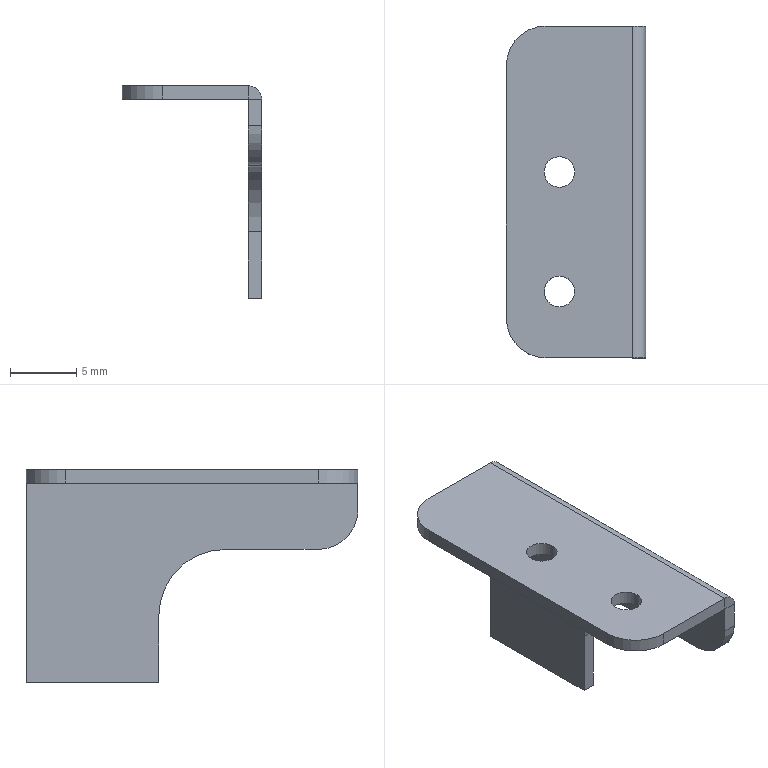Part | SolidWorks | features ICE 2, Fillet 1, FlatPattern 1, SMBaseFlange 1, SheetMetal 1 | 1 solid | 23 faces | box 10.5 x 25 x 16 mm | volume 473.396 mm3 | plane 14 | cylinder 9 | commonest cylinder face diameters 2.3 x4 6 x3 2 x1 10 x1
STEP:
#1=CARTESIAN_POINT('',(-6.65,14.,0.));
#2=VERTEX_POINT('',#1);
#3=CARTESIAN_POINT('',(-4.35,14.,0.));
#4=VERTEX_POINT('',#3);
#5=CARTESIAN_POINT('',(-5.5,14.,0.));
#6=DIRECTION('',(0.,0.,1.));
#7=DIRECTION('',(1.,0.,0.));
#8=AXIS2_PLACEMENT_3D('',#5,#6,#7);
#9=CIRCLE('',#8,1.15);
#10=EDGE_CURVE('',#2,#4,#9,.T.);
#11=ORIENTED_EDGE('',*,*,#10,.F.);
#12=CARTESIAN_POINT('',(-6.65,14.,1.));
#13=VERTEX_POINT('',#12);
#14=CARTESIAN_POINT('',(-6.65,14.,-9.));
#15=DIRECTION('',(0.,0.,1.));
#16=VECTOR('',#15,1000.);
#17=LINE('',#14,#16);
#18=EDGE_CURVE('',#2,#13,#17,.T.);
#19=ORIENTED_EDGE('',*,*,#18,.T.);
#20=CARTESIAN_POINT('',(-4.35,14.,1.));
#21=VERTEX_POINT('',#20);
#22=CARTESIAN_POINT('',(-5.5,14.,1.));
#23=DIRECTION('',(0.,0.,1.));
#24=DIRECTION('',(1.,0.,0.));
#25=AXIS2_PLACEMENT_3D('',#22,#23,#24);
#26=CIRCLE('',#25,1.15);
#27=EDGE_CURVE('',#13,#21,#26,.T.);
#28=ORIENTED_EDGE('',*,*,#27,.T.);
#29=CARTESIAN_POINT('',(-4.35,14.,-9.));
#30=DIRECTION('',(0.,0.,1.));
#31=VECTOR('',#30,1000.);
#32=LINE('',#29,#31);
#33=EDGE_CURVE('',#4,#21,#32,.T.);
#34=ORIENTED_EDGE('',*,*,#33,.F.);
#35=EDGE_LOOP('',(#11,#19,#28,#34));
#36=FACE_OUTER_BOUND('',#35,.T.);
#37=CARTESIAN_POINT('',(-5.5,14.,-9.));
#38=DIRECTION('',(0.,0.,1.));
#39=DIRECTION('',(1.,0.,0.));
#40=AXIS2_PLACEMENT_3D('',#37,#38,#39);
#41=CYLINDRICAL_SURFACE('',#40,1.15);
#42=ADVANCED_FACE('',(#36),#41,.F.);
#43=CARTESIAN_POINT('',(-6.65,5.,0.));
#44=VERTEX_POINT('',#43);
#45=CARTESIAN_POINT('',(-4.35,5.,0.));
#46=VERTEX_POINT('',#45);
#47=CARTESIAN_POINT('',(-5.5,5.,0.));
#48=DIRECTION('',(0.,0.,1.));
#49=DIRECTION('',(1.,0.,0.));
#50=AXIS2_PLACEMENT_3D('',#47,#48,#49);
#51=CIRCLE('',#50,1.15);
#52=EDGE_CURVE('',#44,#46,#51,.T.);
#53=ORIENTED_EDGE('',*,*,#52,.F.);
#54=CARTESIAN_POINT('',(-6.65,5.,1.));
#55=VERTEX_POINT('',#54);
#56=CARTESIAN_POINT('',(-6.65,5.,-9.));
#57=DIRECTION('',(0.,0.,1.));
#58=VECTOR('',#57,1000.);
#59=LINE('',#56,#58);
#60=EDGE_CURVE('',#44,#55,#59,.T.);
#61=ORIENTED_EDGE('',*,*,#60,.T.);
#62=CARTESIAN_POINT('',(-4.35,5.,1.));
#63=VERTEX_POINT('',#62);
#64=CARTESIAN_POINT('',(-5.5,5.,1.));
#65=DIRECTION('',(0.,0.,1.));
#66=DIRECTION('',(1.,0.,0.));
#67=AXIS2_PLACEMENT_3D('',#64,#65,#66);
#68=CIRCLE('',#67,1.15);
#69=EDGE_CURVE('',#55,#63,#68,.T.);
#70=ORIENTED_EDGE('',*,*,#69,.T.);
#71=CARTESIAN_POINT('',(-4.35,5.,-9.));
#72=DIRECTION('',(0.,0.,1.));
#73=VECTOR('',#72,1000.);
#74=LINE('',#71,#73);
#75=EDGE_CURVE('',#46,#63,#74,.T.);
#76=ORIENTED_EDGE('',*,*,#75,.F.);
#77=EDGE_LOOP('',(#53,#61,#70,#76));
#78=FACE_OUTER_BOUND('',#77,.T.);
#79=CARTESIAN_POINT('',(-5.5,5.,-9.));
#80=DIRECTION('',(0.,0.,1.));
#81=DIRECTION('',(1.,0.,0.));
#82=AXIS2_PLACEMENT_3D('',#79,#80,#81);
#83=CYLINDRICAL_SURFACE('',#82,1.15);
#84=ADVANCED_FACE('',(#78),#83,.F.);
#85=CARTESIAN_POINT('',(0.,0.,-2.));
#86=VERTEX_POINT('',#85);
#87=CARTESIAN_POINT('',(0.,0.,0.));
#88=VERTEX_POINT('',#87);
#89=CARTESIAN_POINT('',(0.,0.,-15.));
#90=DIRECTION('',(0.,0.,1.));
#91=VECTOR('',#90,1000.);
#92=LINE('',#89,#91);
#93=EDGE_CURVE('',#86,#88,#92,.T.);
#94=ORIENTED_EDGE('',*,*,#93,.F.);
#95=CARTESIAN_POINT('',(1.,0.,-2.));
#96=VERTEX_POINT('',#95);
#97=CARTESIAN_POINT('',(1.,0.,-2.));
#98=DIRECTION('',(1.,0.,0.));
#99=VECTOR('',#98,1000.);
#100=LINE('',#97,#99);
#101=EDGE_CURVE('',#86,#96,#100,.T.);
#102=ORIENTED_EDGE('',*,*,#101,.T.);
#103=CARTESIAN_POINT('',(1.,0.,0.));
#104=VERTEX_POINT('',#103);
#105=CARTESIAN_POINT('',(1.,0.,-15.));
#106=DIRECTION('',(0.,0.,1.));
#107=VECTOR('',#106,1000.);
#108=LINE('',#105,#107);
#109=EDGE_CURVE('',#96,#104,#108,.T.);
#110=ORIENTED_EDGE('',*,*,#109,.T.);
#111=CARTESIAN_POINT('',(0.,0.,0.));
#112=DIRECTION('',(1.,0.,0.));
#113=VECTOR('',#112,1000.);
#114=LINE('',#111,#113);
#115=EDGE_CURVE('',#88,#104,#114,.T.);
#116=ORIENTED_EDGE('',*,*,#115,.F.);
#117=EDGE_LOOP('',(#94,#102,#110,#116));
#118=FACE_OUTER_BOUND('',#117,.T.);
#119=CARTESIAN_POINT('',(0.,0.,0.));
#120=DIRECTION('',(0.,-1.,0.));
#121=DIRECTION('',(0.,0.,-1.));
#122=AXIS2_PLACEMENT_3D('',#119,#120,#121);
#123=PLANE('',#122);
#124=ADVANCED_FACE('',(#118),#123,.T.);
#125=CARTESIAN_POINT('',(0.,0.,1.));
#126=VERTEX_POINT('',#125);
#127=CARTESIAN_POINT('',(0.,0.,0.));
#128=DIRECTION('',(0.,0.,1.));
#129=VECTOR('',#128,1000.);
#130=LINE('',#127,#129);
#131=EDGE_CURVE('',#88,#126,#130,.T.);
#132=ORIENTED_EDGE('',*,*,#131,.F.);
#133=ORIENTED_EDGE('',*,*,#115,.T.);
#134=CARTESIAN_POINT('',(0.,0.,0.));
#135=DIRECTION('',(0.,-1.,0.));
#136=DIRECTION('',(0.,0.,-1.));
#137=AXIS2_PLACEMENT_3D('',#134,#135,#136);
#138=CIRCLE('',#137,1.);
#139=EDGE_CURVE('',#104,#126,#138,.T.);
#140=ORIENTED_EDGE('',*,*,#139,.T.);
#141=EDGE_LOOP('',(#132,#133,#140));
#142=FACE_OUTER_BOUND('',#141,.T.);
#143=CARTESIAN_POINT('',(0.,0.,0.));
#144=DIRECTION('',(0.,-1.,0.));
#145=DIRECTION('',(0.,0.,-1.));
#146=AXIS2_PLACEMENT_3D('',#143,#144,#145);
#147=PLANE('',#146);
#148=ADVANCED_FACE('',(#142),#147,.T.);
#149=CARTESIAN_POINT('',(0.,25.,0.));
#150=VERTEX_POINT('',#149);
#151=CARTESIAN_POINT('',(-6.5,25.,0.));
#152=VERTEX_POINT('',#151);
#153=CARTESIAN_POINT('',(0.,25.,0.));
#154=DIRECTION('',(-1.,0.,0.));
#155=VECTOR('',#154,1000.);
#156=LINE('',#153,#155);
#157=EDGE_CURVE('',#150,#152,#156,.T.);
#158=ORIENTED_EDGE('',*,*,#157,.T.);
#159=CARTESIAN_POINT('',(-6.5,25.,1.));
#160=VERTEX_POINT('',#159);
#161=CARTESIAN_POINT('',(-6.5,25.,0.));
#162=DIRECTION('',(0.,0.,1.));
#163=VECTOR('',#162,1000.);
#164=LINE('',#161,#163);
#165=EDGE_CURVE('',#152,#160,#164,.T.);
#166=ORIENTED_EDGE('',*,*,#165,.T.);
#167=CARTESIAN_POINT('',(0.,25.,1.));
#168=VERTEX_POINT('',#167);
#169=CARTESIAN_POINT('',(0.,25.,1.));
#170=DIRECTION('',(-1.,0.,0.));
#171=VECTOR('',#170,1000.);
#172=LINE('',#169,#171);
#173=EDGE_CURVE('',#168,#160,#172,.T.);
#174=ORIENTED_EDGE('',*,*,#173,.F.);
#175=CARTESIAN_POINT('',(0.,25.,0.));
#176=DIRECTION('',(0.,0.,1.));
#177=VECTOR('',#176,1000.);
#178=LINE('',#175,#177);
#179=EDGE_CURVE('',#150,#168,#178,.T.);
#180=ORIENTED_EDGE('',*,*,#179,.F.);
#181=EDGE_LOOP('',(#158,#166,#174,#180));
#182=FACE_OUTER_BOUND('',#181,.T.);
#183=CARTESIAN_POINT('',(0.,25.,0.));
#184=DIRECTION('',(0.,1.,0.));
#185=DIRECTION('',(0.,0.,1.));
#186=AXIS2_PLACEMENT_3D('',#183,#184,#185);
#187=PLANE('',#186);
#188=ADVANCED_FACE('',(#182),#187,.T.);
#189=CARTESIAN_POINT('',(1.,25.,0.));
#190=VERTEX_POINT('',#189);
#191=CARTESIAN_POINT('',(0.,25.,0.));
#192=DIRECTION('',(1.,0.,0.));
#193=VECTOR('',#192,1000.);
#194=LINE('',#191,#193);
#195=EDGE_CURVE('',#150,#190,#194,.T.);
#196=ORIENTED_EDGE('',*,*,#195,.F.);
#197=ORIENTED_EDGE('',*,*,#179,.T.);
#198=CARTESIAN_POINT('',(0.,25.,0.));
#199=DIRECTION('',(0.,1.,0.));
#200=DIRECTION('',(0.,0.,-1.));
#201=AXIS2_PLACEMENT_3D('',#198,#199,#200);
#202=CIRCLE('',#201,1.);
#203=EDGE_CURVE('',#168,#190,#202,.T.);
#204=ORIENTED_EDGE('',*,*,#203,.T.);
#205=EDGE_LOOP('',(#196,#197,#204));
#206=FACE_OUTER_BOUND('',#205,.T.);
#207=CARTESIAN_POINT('',(0.,25.,0.));
#208=DIRECTION('',(0.,1.,0.));
#209=DIRECTION('',(0.,0.,1.));
#210=AXIS2_PLACEMENT_3D('',#207,#208,#209);
#211=PLANE('',#210);
#212=ADVANCED_FACE('',(#206),#211,.T.);
#213=CARTESIAN_POINT('',(-5.5,14.,0.));
#214=DIRECTION('',(0.,0.,1.));
#215=DIRECTION('',(1.,0.,0.));
#216=AXIS2_PLACEMENT_3D('',#213,#214,#215);
#217=CIRCLE('',#216,1.15);
#218=EDGE_CURVE('',#4,#2,#217,.T.);
#219=ORIENTED_EDGE('',*,*,#218,.T.);
#220=ORIENTED_EDGE('',*,*,#10,.T.);
#221=EDGE_LOOP('',(#219,#220));
#222=FACE_BOUND('',#221,.T.);
#223=CARTESIAN_POINT('',(-5.5,5.,0.));
#224=DIRECTION('',(0.,0.,1.));
#225=DIRECTION('',(1.,0.,0.));
#226=AXIS2_PLACEMENT_3D('',#223,#224,#225);
#227=CIRCLE('',#226,1.15);
#228=EDGE_CURVE('',#46,#44,#227,.T.);
#229=ORIENTED_EDGE('',*,*,#228,.T.);
#230=ORIENTED_EDGE('',*,*,#52,.T.);
#231=EDGE_LOOP('',(#229,#230));
#232=FACE_BOUND('',#231,.T.);
#233=CARTESIAN_POINT('',(-9.5,22.,0.));
#234=VERTEX_POINT('',#233);
#235=CARTESIAN_POINT('',(-9.5,3.,0.));
#236=VERTEX_POINT('',#235);
#237=CARTESIAN_POINT('',(-9.5,25.,0.));
#238=DIRECTION('',(0.,-1.,0.));
#239=VECTOR('',#238,1000.);
#240=LINE('',#237,#239);
#241=EDGE_CURVE('',#234,#236,#240,.T.);
#242=ORIENTED_EDGE('',*,*,#241,.F.);
#243=CARTESIAN_POINT('',(-6.5,22.,0.));
#244=DIRECTION('',(0.,0.,-1.));
#245=DIRECTION('',(1.,0.,0.));
#246=AXIS2_PLACEMENT_3D('',#243,#244,#245);
#247=CIRCLE('',#246,3.);
#248=EDGE_CURVE('',#234,#152,#247,.T.);
#249=ORIENTED_EDGE('',*,*,#248,.T.);
#250=ORIENTED_EDGE('',*,*,#157,.F.);
#251=CARTESIAN_POINT('',(0.,25.,0.));
#252=DIRECTION('',(0.,-1.,0.));
#253=VECTOR('',#252,1000.);
#254=LINE('',#251,#253);
#255=EDGE_CURVE('',#150,#88,#254,.T.);
#256=ORIENTED_EDGE('',*,*,#255,.T.);
#257=CARTESIAN_POINT('',(-6.5,0.,0.));
#258=VERTEX_POINT('',#257);
#259=CARTESIAN_POINT('',(0.,0.,0.));
#260=DIRECTION('',(-1.,0.,0.));
#261=VECTOR('',#260,1000.);
#262=LINE('',#259,#261);
#263=EDGE_CURVE('',#88,#258,#262,.T.);
#264=ORIENTED_EDGE('',*,*,#263,.T.);
#265=CARTESIAN_POINT('',(-6.5,3.,0.));
#266=DIRECTION('',(0.,0.,-1.));
#267=DIRECTION('',(1.,0.,0.));
#268=AXIS2_PLACEMENT_3D('',#265,#266,#267);
#269=CIRCLE('',#268,3.);
#270=EDGE_CURVE('',#258,#236,#269,.T.);
#271=ORIENTED_EDGE('',*,*,#270,.T.);
#272=EDGE_LOOP('',(#242,#249,#250,#256,#264,#271));
#273=FACE_OUTER_BOUND('',#272,.T.);
#274=CARTESIAN_POINT('',(0.,25.,0.));
#275=DIRECTION('',(0.,0.,1.));
#276=DIRECTION('',(1.,0.,0.));
#277=AXIS2_PLACEMENT_3D('',#274,#275,#276);
#278=PLANE('',#277);
#279=ADVANCED_FACE('',(#222,#232,#273),#278,.F.);
#280=CARTESIAN_POINT('',(-9.5,22.,1.));
#281=VERTEX_POINT('',#280);
#282=CARTESIAN_POINT('',(-9.5,3.,1.));
#283=VERTEX_POINT('',#282);
#284=CARTESIAN_POINT('',(-9.5,25.,1.));
#285=DIRECTION('',(0.,-1.,0.));
#286=VECTOR('',#285,1000.);
#287=LINE('',#284,#286);
#288=EDGE_CURVE('',#281,#283,#287,.T.);
#289=ORIENTED_EDGE('',*,*,#288,.F.);
#290=CARTESIAN_POINT('',(-9.5,22.,1.));
#291=DIRECTION('',(0.,0.,-1.));
#292=VECTOR('',#291,1000.);
#293=LINE('',#290,#292);
#294=EDGE_CURVE('',#281,#234,#293,.T.);
#295=ORIENTED_EDGE('',*,*,#294,.T.);
#296=ORIENTED_EDGE('',*,*,#241,.T.);
#297=CARTESIAN_POINT('',(-9.5,3.,1.));
#298=DIRECTION('',(0.,0.,1.));
#299=VECTOR('',#298,1000.);
#300=LINE('',#297,#299);
#301=EDGE_CURVE('',#236,#283,#300,.T.);
#302=ORIENTED_EDGE('',*,*,#301,.T.);
#303=EDGE_LOOP('',(#289,#295,#296,#302));
#304=FACE_OUTER_BOUND('',#303,.T.);
#305=CARTESIAN_POINT('',(-9.5,25.,1.));
#306=DIRECTION('',(-1.,0.,0.));
#307=DIRECTION('',(0.,0.,1.));
#308=AXIS2_PLACEMENT_3D('',#305,#306,#307);
#309=PLANE('',#308);
#310=ADVANCED_FACE('',(#304),#309,.T.);
#311=CARTESIAN_POINT('',(-5.5,14.,1.));
#312=DIRECTION('',(0.,0.,1.));
#313=DIRECTION('',(1.,0.,0.));
#314=AXIS2_PLACEMENT_3D('',#311,#312,#313);
#315=CIRCLE('',#314,1.15);
#316=EDGE_CURVE('',#21,#13,#315,.T.);
#317=ORIENTED_EDGE('',*,*,#316,.F.);
#318=ORIENTED_EDGE('',*,*,#27,.F.);
#319=EDGE_LOOP('',(#317,#318));
#320=FACE_BOUND('',#319,.T.);
#321=CARTESIAN_POINT('',(-5.5,5.,1.));
#322=DIRECTION('',(0.,0.,1.));
#323=DIRECTION('',(1.,0.,0.));
#324=AXIS2_PLACEMENT_3D('',#321,#322,#323);
#325=CIRCLE('',#324,1.15);
#326=EDGE_CURVE('',#63,#55,#325,.T.);
#327=ORIENTED_EDGE('',*,*,#326,.F.);
#328=ORIENTED_EDGE('',*,*,#69,.F.);
#329=EDGE_LOOP('',(#327,#328));
#330=FACE_BOUND('',#329,.T.);
#331=ORIENTED_EDGE('',*,*,#173,.T.);
#332=CARTESIAN_POINT('',(-6.5,22.,1.));
#333=DIRECTION('',(0.,0.,1.));
#334=DIRECTION('',(1.,0.,0.));
#335=AXIS2_PLACEMENT_3D('',#332,#333,#334);
#336=CIRCLE('',#335,3.);
#337=EDGE_CURVE('',#160,#281,#336,.T.);
#338=ORIENTED_EDGE('',*,*,#337,.T.);
#339=ORIENTED_EDGE('',*,*,#288,.T.);
#340=CARTESIAN_POINT('',(-6.5,0.,1.));
#341=VERTEX_POINT('',#340);
#342=CARTESIAN_POINT('',(-6.5,3.,1.));
#343=DIRECTION('',(0.,0.,1.));
#344=DIRECTION('',(1.,0.,0.));
#345=AXIS2_PLACEMENT_3D('',#342,#343,#344);
#346=CIRCLE('',#345,3.);
#347=EDGE_CURVE('',#283,#341,#346,.T.);
#348=ORIENTED_EDGE('',*,*,#347,.T.);
#349=CARTESIAN_POINT('',(0.,0.,1.));
#350=DIRECTION('',(-1.,0.,0.));
#351=VECTOR('',#350,1000.);
#352=LINE('',#349,#351);
#353=EDGE_CURVE('',#126,#341,#352,.T.);
#354=ORIENTED_EDGE('',*,*,#353,.F.);
#355=CARTESIAN_POINT('',(0.,25.,1.));
#356=DIRECTION('',(0.,1.,0.));
#357=VECTOR('',#356,1000.);
#358=LINE('',#355,#357);
#359=EDGE_CURVE('',#126,#168,#358,.T.);
#360=ORIENTED_EDGE('',*,*,#359,.T.);
#361=EDGE_LOOP('',(#331,#338,#339,#348,#354,#360));
#362=FACE_OUTER_BOUND('',#361,.T.);
#363=CARTESIAN_POINT('',(0.,25.,1.));
#364=DIRECTION('',(0.,0.,1.));
#365=DIRECTION('',(1.,0.,0.));
#366=AXIS2_PLACEMENT_3D('',#363,#364,#365);
#367=PLANE('',#366);
#368=ADVANCED_FACE('',(#320,#330,#362),#367,.T.);
#369=ORIENTED_EDGE('',*,*,#109,.F.);
#370=CARTESIAN_POINT('',(1.,3.,-5.));
#371=VERTEX_POINT('',#370);
#372=CARTESIAN_POINT('',(1.,3.,-2.));
#373=DIRECTION('',(1.,0.,0.));
#374=DIRECTION('',(0.,0.,-1.));
#375=AXIS2_PLACEMENT_3D('',#372,#373,#374);
#376=CIRCLE('',#375,3.);
#377=EDGE_CURVE('',#96,#371,#376,.T.);
#378=ORIENTED_EDGE('',*,*,#377,.T.);
#379=CARTESIAN_POINT('',(1.,10.,-5.));
#380=VERTEX_POINT('',#379);
#381=CARTESIAN_POINT('',(1.,0.,-5.));
#382=DIRECTION('',(0.,-1.,0.));
#383=VECTOR('',#382,1000.);
#384=LINE('',#381,#383);
#385=EDGE_CURVE('',#380,#371,#384,.T.);
#386=ORIENTED_EDGE('',*,*,#385,.F.);
#387=CARTESIAN_POINT('',(1.,15.,-10.));
#388=VERTEX_POINT('',#387);
#389=CARTESIAN_POINT('',(1.,10.,-10.));
#390=DIRECTION('',(1.,0.,0.));
#391=DIRECTION('',(0.,0.,-1.));
#392=AXIS2_PLACEMENT_3D('',#389,#390,#391);
#393=CIRCLE('',#392,5.);
#394=EDGE_CURVE('',#388,#380,#393,.T.);
#395=ORIENTED_EDGE('',*,*,#394,.F.);
#396=CARTESIAN_POINT('',(1.,15.,-15.));
#397=VERTEX_POINT('',#396);
#398=CARTESIAN_POINT('',(1.,15.,-15.));
#399=DIRECTION('',(0.,0.,1.));
#400=VECTOR('',#399,1000.);
#401=LINE('',#398,#400);
#402=EDGE_CURVE('',#397,#388,#401,.T.);
#403=ORIENTED_EDGE('',*,*,#402,.F.);
#404=CARTESIAN_POINT('',(1.,25.,-15.));
#405=VERTEX_POINT('',#404);
#406=CARTESIAN_POINT('',(1.,25.,-15.));
#407=DIRECTION('',(0.,-1.,0.));
#408=VECTOR('',#407,1000.);
#409=LINE('',#406,#408);
#410=EDGE_CURVE('',#405,#397,#409,.T.);
#411=ORIENTED_EDGE('',*,*,#410,.F.);
#412=CARTESIAN_POINT('',(1.,25.,-15.));
#413=DIRECTION('',(0.,0.,1.));
#414=VECTOR('',#413,1000.);
#415=LINE('',#412,#414);
#416=EDGE_CURVE('',#405,#190,#415,.T.);
#417=ORIENTED_EDGE('',*,*,#416,.T.);
#418=CARTESIAN_POINT('',(1.,25.,0.));
#419=DIRECTION('',(0.,-1.,0.));
#420=VECTOR('',#419,1000.);
#421=LINE('',#418,#420);
#422=EDGE_CURVE('',#190,#104,#421,.T.);
#423=ORIENTED_EDGE('',*,*,#422,.T.);
#424=EDGE_LOOP('',(#369,#378,#386,#395,#403,#411,#417,#423));
#425=FACE_OUTER_BOUND('',#424,.T.);
#426=CARTESIAN_POINT('',(1.,25.,-15.));
#427=DIRECTION('',(1.,0.,0.));
#428=DIRECTION('',(0.,0.,-1.));
#429=AXIS2_PLACEMENT_3D('',#426,#427,#428);
#430=PLANE('',#429);
#431=ADVANCED_FACE('',(#425),#430,.T.);
#432=CARTESIAN_POINT('',(0.,15.,-15.));
#433=VERTEX_POINT('',#432);
#434=CARTESIAN_POINT('',(-9.,15.,-15.));
#435=DIRECTION('',(1.,0.,0.));
#436=VECTOR('',#435,1000.);
#437=LINE('',#434,#436);
#438=EDGE_CURVE('',#433,#397,#437,.T.);
#439=ORIENTED_EDGE('',*,*,#438,.F.);
#440=CARTESIAN_POINT('',(0.,25.,-15.));
#441=VERTEX_POINT('',#440);
#442=CARTESIAN_POINT('',(0.,25.,-15.));
#443=DIRECTION('',(0.,-1.,0.));
#444=VECTOR('',#443,1000.);
#445=LINE('',#442,#444);
#446=EDGE_CURVE('',#441,#433,#445,.T.);
#447=ORIENTED_EDGE('',*,*,#446,.F.);
#448=CARTESIAN_POINT('',(0.,25.,-15.));
#449=DIRECTION('',(1.,0.,0.));
#450=VECTOR('',#449,1000.);
#451=LINE('',#448,#450);
#452=EDGE_CURVE('',#441,#405,#451,.T.);
#453=ORIENTED_EDGE('',*,*,#452,.T.);
#454=ORIENTED_EDGE('',*,*,#410,.T.);
#455=EDGE_LOOP('',(#439,#447,#453,#454));
#456=FACE_OUTER_BOUND('',#455,.T.);
#457=CARTESIAN_POINT('',(0.,25.,-15.));
#458=DIRECTION('',(0.,0.,-1.));
#459=DIRECTION('',(-1.,0.,0.));
#460=AXIS2_PLACEMENT_3D('',#457,#458,#459);
#461=PLANE('',#460);
#462=ADVANCED_FACE('',(#456),#461,.T.);
#463=CARTESIAN_POINT('',(0.,10.,-5.));
#464=VERTEX_POINT('',#463);
#465=CARTESIAN_POINT('',(0.,3.,-5.));
#466=VERTEX_POINT('',#465);
#467=CARTESIAN_POINT('',(0.,25.,-5.));
#468=DIRECTION('',(0.,-1.,0.));
#469=VECTOR('',#468,1000.);
#470=LINE('',#467,#469);
#471=EDGE_CURVE('',#464,#466,#470,.T.);
#472=ORIENTED_EDGE('',*,*,#471,.T.);
#473=CARTESIAN_POINT('',(0.,3.,-2.));
#474=DIRECTION('',(-1.,0.,0.));
#475=DIRECTION('',(0.,0.,-1.));
#476=AXIS2_PLACEMENT_3D('',#473,#474,#475);
#477=CIRCLE('',#476,3.);
#478=EDGE_CURVE('',#466,#86,#477,.T.);
#479=ORIENTED_EDGE('',*,*,#478,.T.);
#480=ORIENTED_EDGE('',*,*,#93,.T.);
#481=ORIENTED_EDGE('',*,*,#255,.F.);
#482=CARTESIAN_POINT('',(0.,25.,-15.));
#483=DIRECTION('',(0.,0.,1.));
#484=VECTOR('',#483,1000.);
#485=LINE('',#482,#484);
#486=EDGE_CURVE('',#441,#150,#485,.T.);
#487=ORIENTED_EDGE('',*,*,#486,.F.);
#488=ORIENTED_EDGE('',*,*,#446,.T.);
#489=CARTESIAN_POINT('',(0.,15.,-10.));
#490=VERTEX_POINT('',#489);
#491=CARTESIAN_POINT('',(0.,15.,-15.));
#492=DIRECTION('',(0.,0.,1.));
#493=VECTOR('',#492,1000.);
#494=LINE('',#491,#493);
#495=EDGE_CURVE('',#433,#490,#494,.T.);
#496=ORIENTED_EDGE('',*,*,#495,.T.);
#497=CARTESIAN_POINT('',(0.,10.,-10.));
#498=DIRECTION('',(1.,0.,0.));
#499=DIRECTION('',(0.,0.,-1.));
#500=AXIS2_PLACEMENT_3D('',#497,#498,#499);
#501=CIRCLE('',#500,5.);
#502=EDGE_CURVE('',#490,#464,#501,.T.);
#503=ORIENTED_EDGE('',*,*,#502,.T.);
#504=EDGE_LOOP('',(#472,#479,#480,#481,#487,#488,#496,#503));
#505=FACE_OUTER_BOUND('',#504,.T.);
#506=CARTESIAN_POINT('',(0.,25.,-15.));
#507=DIRECTION('',(1.,0.,0.));
#508=DIRECTION('',(0.,0.,-1.));
#509=AXIS2_PLACEMENT_3D('',#506,#507,#508);
#510=PLANE('',#509);
#511=ADVANCED_FACE('',(#505),#510,.F.);
#512=ORIENTED_EDGE('',*,*,#486,.T.);
#513=ORIENTED_EDGE('',*,*,#195,.T.);
#514=ORIENTED_EDGE('',*,*,#416,.F.);
#515=ORIENTED_EDGE('',*,*,#452,.F.);
#516=EDGE_LOOP('',(#512,#513,#514,#515));
#517=FACE_OUTER_BOUND('',#516,.T.);
#518=CARTESIAN_POINT('',(0.,25.,0.));
#519=DIRECTION('',(0.,-1.,0.));
#520=DIRECTION('',(-1.,0.,0.));
#521=AXIS2_PLACEMENT_3D('',#518,#519,#520);
#522=PLANE('',#521);
#523=ADVANCED_FACE('',(#517),#522,.F.);
#524=ORIENTED_EDGE('',*,*,#353,.T.);
#525=CARTESIAN_POINT('',(-6.5,0.,0.));
#526=DIRECTION('',(0.,0.,-1.));
#527=VECTOR('',#526,1000.);
#528=LINE('',#525,#527);
#529=EDGE_CURVE('',#341,#258,#528,.T.);
#530=ORIENTED_EDGE('',*,*,#529,.T.);
#531=ORIENTED_EDGE('',*,*,#263,.F.);
#532=ORIENTED_EDGE('',*,*,#131,.T.);
#533=EDGE_LOOP('',(#524,#530,#531,#532));
#534=FACE_OUTER_BOUND('',#533,.T.);
#535=CARTESIAN_POINT('',(0.,0.,0.));
#536=DIRECTION('',(0.,-1.,0.));
#537=DIRECTION('',(-1.,0.,0.));
#538=AXIS2_PLACEMENT_3D('',#535,#536,#537);
#539=PLANE('',#538);
#540=ADVANCED_FACE('',(#534),#539,.T.);
#541=ORIENTED_EDGE('',*,*,#203,.F.);
#542=ORIENTED_EDGE('',*,*,#359,.F.);
#543=ORIENTED_EDGE('',*,*,#139,.F.);
#544=ORIENTED_EDGE('',*,*,#422,.F.);
#545=EDGE_LOOP('',(#541,#542,#543,#544));
#546=FACE_OUTER_BOUND('',#545,.T.);
#547=CARTESIAN_POINT('',(0.,25.,0.));
#548=DIRECTION('',(0.,-1.,0.));
#549=DIRECTION('',(0.,0.,-1.));
#550=AXIS2_PLACEMENT_3D('',#547,#548,#549);
#551=CYLINDRICAL_SURFACE('',#550,1.);
#552=ADVANCED_FACE('',(#546),#551,.T.);
#553=ORIENTED_EDGE('',*,*,#60,.F.);
#554=ORIENTED_EDGE('',*,*,#228,.F.);
#555=ORIENTED_EDGE('',*,*,#75,.T.);
#556=ORIENTED_EDGE('',*,*,#326,.T.);
#557=EDGE_LOOP('',(#553,#554,#555,#556));
#558=FACE_OUTER_BOUND('',#557,.T.);
#559=CARTESIAN_POINT('',(-5.5,5.,-9.));
#560=DIRECTION('',(0.,0.,1.));
#561=DIRECTION('',(1.,0.,0.));
#562=AXIS2_PLACEMENT_3D('',#559,#560,#561);
#563=CYLINDRICAL_SURFACE('',#562,1.15);
#564=ADVANCED_FACE('',(#558),#563,.F.);
#565=ORIENTED_EDGE('',*,*,#18,.F.);
#566=ORIENTED_EDGE('',*,*,#218,.F.);
#567=ORIENTED_EDGE('',*,*,#33,.T.);
#568=ORIENTED_EDGE('',*,*,#316,.T.);
#569=EDGE_LOOP('',(#565,#566,#567,#568));
#570=FACE_OUTER_BOUND('',#569,.T.);
#571=CARTESIAN_POINT('',(-5.5,14.,-9.));
#572=DIRECTION('',(0.,0.,1.));
#573=DIRECTION('',(1.,0.,0.));
#574=AXIS2_PLACEMENT_3D('',#571,#572,#573);
#575=CYLINDRICAL_SURFACE('',#574,1.15);
#576=ADVANCED_FACE('',(#570),#575,.F.);
#577=ORIENTED_EDGE('',*,*,#385,.T.);
#578=CARTESIAN_POINT('',(0.,3.,-5.));
#579=DIRECTION('',(-1.,0.,0.));
#580=VECTOR('',#579,1000.);
#581=LINE('',#578,#580);
#582=EDGE_CURVE('',#371,#466,#581,.T.);
#583=ORIENTED_EDGE('',*,*,#582,.T.);
#584=ORIENTED_EDGE('',*,*,#471,.F.);
#585=CARTESIAN_POINT('',(-9.,10.,-5.));
#586=DIRECTION('',(1.,0.,0.));
#587=VECTOR('',#586,1000.);
#588=LINE('',#585,#587);
#589=EDGE_CURVE('',#464,#380,#588,.T.);
#590=ORIENTED_EDGE('',*,*,#589,.T.);
#591=EDGE_LOOP('',(#577,#583,#584,#590));
#592=FACE_OUTER_BOUND('',#591,.T.);
#593=CARTESIAN_POINT('',(-9.,0.,-5.));
#594=DIRECTION('',(0.,0.,1.));
#595=DIRECTION('',(1.,0.,0.));
#596=AXIS2_PLACEMENT_3D('',#593,#594,#595);
#597=PLANE('',#596);
#598=ADVANCED_FACE('',(#592),#597,.F.);
#599=CARTESIAN_POINT('',(-9.,15.,-10.));
#600=DIRECTION('',(1.,0.,0.));
#601=VECTOR('',#600,1000.);
#602=LINE('',#599,#601);
#603=EDGE_CURVE('',#490,#388,#602,.T.);
#604=ORIENTED_EDGE('',*,*,#603,.T.);
#605=ORIENTED_EDGE('',*,*,#394,.T.);
#606=ORIENTED_EDGE('',*,*,#589,.F.);
#607=ORIENTED_EDGE('',*,*,#502,.F.);
#608=EDGE_LOOP('',(#604,#605,#606,#607));
#609=FACE_OUTER_BOUND('',#608,.T.);
#610=CARTESIAN_POINT('',(-9.,10.,-10.));
#611=DIRECTION('',(1.,0.,0.));
#612=DIRECTION('',(0.,0.,-1.));
#613=AXIS2_PLACEMENT_3D('',#610,#611,#612);
#614=CYLINDRICAL_SURFACE('',#613,5.);
#615=ADVANCED_FACE('',(#609),#614,.F.);
#616=ORIENTED_EDGE('',*,*,#438,.T.);
#617=ORIENTED_EDGE('',*,*,#402,.T.);
#618=ORIENTED_EDGE('',*,*,#603,.F.);
#619=ORIENTED_EDGE('',*,*,#495,.F.);
#620=EDGE_LOOP('',(#616,#617,#618,#619));
#621=FACE_OUTER_BOUND('',#620,.T.);
#622=CARTESIAN_POINT('',(-9.,15.,-15.));
#623=DIRECTION('',(0.,1.,0.));
#624=DIRECTION('',(0.,0.,1.));
#625=AXIS2_PLACEMENT_3D('',#622,#623,#624);
#626=PLANE('',#625);
#627=ADVANCED_FACE('',(#621),#626,.F.);
#628=ORIENTED_EDGE('',*,*,#337,.F.);
#629=ORIENTED_EDGE('',*,*,#165,.F.);
#630=ORIENTED_EDGE('',*,*,#248,.F.);
#631=ORIENTED_EDGE('',*,*,#294,.F.);
#632=EDGE_LOOP('',(#628,#629,#630,#631));
#633=FACE_OUTER_BOUND('',#632,.T.);
#634=CARTESIAN_POINT('',(-6.5,22.,1.));
#635=DIRECTION('',(0.,0.,-1.));
#636=DIRECTION('',(-1.,0.,0.));
#637=AXIS2_PLACEMENT_3D('',#634,#635,#636);
#638=CYLINDRICAL_SURFACE('',#637,3.);
#639=ADVANCED_FACE('',(#633),#638,.T.);
#640=ORIENTED_EDGE('',*,*,#478,.F.);
#641=ORIENTED_EDGE('',*,*,#582,.F.);
#642=ORIENTED_EDGE('',*,*,#377,.F.);
#643=ORIENTED_EDGE('',*,*,#101,.F.);
#644=EDGE_LOOP('',(#640,#641,#642,#643));
#645=FACE_OUTER_BOUND('',#644,.T.);
#646=CARTESIAN_POINT('',(0.,3.,-2.));
#647=DIRECTION('',(-1.,0.,0.));
#648=DIRECTION('',(0.,0.,1.));
#649=AXIS2_PLACEMENT_3D('',#646,#647,#648);
#650=CYLINDRICAL_SURFACE('',#649,3.);
#651=ADVANCED_FACE('',(#645),#650,.T.);
#652=ORIENTED_EDGE('',*,*,#347,.F.);
#653=ORIENTED_EDGE('',*,*,#301,.F.);
#654=ORIENTED_EDGE('',*,*,#270,.F.);
#655=ORIENTED_EDGE('',*,*,#529,.F.);
#656=EDGE_LOOP('',(#652,#653,#654,#655));
#657=FACE_OUTER_BOUND('',#656,.T.);
#658=CARTESIAN_POINT('',(-6.5,3.,0.));
#659=DIRECTION('',(0.,0.,-1.));
#660=DIRECTION('',(-1.,0.,0.));
#661=AXIS2_PLACEMENT_3D('',#658,#659,#660);
#662=CYLINDRICAL_SURFACE('',#661,3.);
#663=ADVANCED_FACE('',(#657),#662,.T.);
#664=CLOSED_SHELL('',(#42,#84,#124,#148,#188,#212,#279,#310,#368,#431,#462,#511,#523,#540,#552,#564,#576,#598,#615,#627,#639,#651,#663));
#665=MANIFOLD_SOLID_BREP('',#664);
#666=CARTESIAN_POINT('',(0.,0.,0.));
#667=DIRECTION('',(0.,0.,1.));
#668=DIRECTION('',(1.,0.,0.));
#669=AXIS2_PLACEMENT_3D('',#666,#667,#668);
#670=(LENGTH_UNIT()NAMED_UNIT(*)SI_UNIT(.MILLI.,.METRE.));
#671=UNCERTAINTY_MEASURE_WITH_UNIT(LENGTH_MEASURE(0.00001),#670,'','');
#672=(NAMED_UNIT(*)PLANE_ANGLE_UNIT()SI_UNIT($,.RADIAN.));
#673=(NAMED_UNIT(*)SI_UNIT($,.STERADIAN.)SOLID_ANGLE_UNIT());
#674=(GEOMETRIC_REPRESENTATION_CONTEXT(3)GLOBAL_UNCERTAINTY_ASSIGNED_CONTEXT((#671))GLOBAL_UNIT_ASSIGNED_CONTEXT((#670,#672,#673))REPRESENTATION_CONTEXT('',''));
#675=ADVANCED_BREP_SHAPE_REPRESENTATION('',(#665,#669),#674);